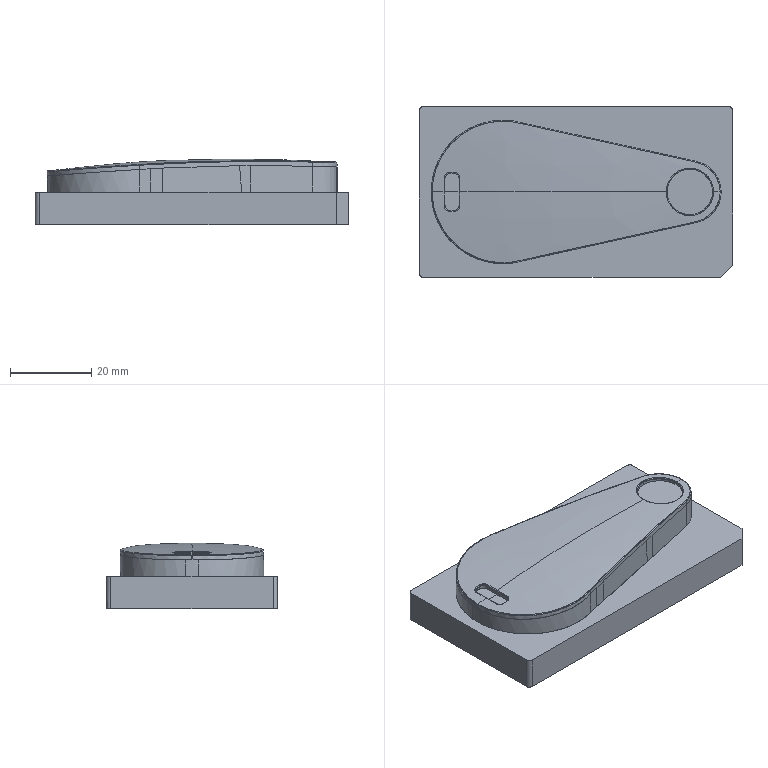NC program | PowerMill | posted with a generic post | part box 77 x 42 x 16.114 mm
Lines 16290 to 17577 of 134652:
N16387 M6
N16388 S18000 M03
N16389 G00 G90 X0.0 Y0.0
N16390 G43 Z9.8037 H28
N16391
N16392 G05 P10000 R4
N16393 X-29.7588 Y2.6569
N16394 Z-1.551
N16395 G01 Z-2.751 F2400.0
N16396 X-29.7423 F4000.0
N16397 G03 X-29.5938 Y2.8054 I0.0 J0.1485
N16398 G01 Y3.0942
N16399 X-29.6282 Y3.438
N16400 X-29.6595 Y3.5057
N16401 X-29.6771 Y3.5369
N16402 X-29.8198 Y3.6917
N16403 X-30.0098 Y3.7818
N16404 X-30.4677 Y3.8359
N16405 X-29.7592 Y2.4875 Z-2.8477
N16406 X-29.7427
N16407 G03 X-29.5942 Y2.636 I0.0 J0.1485
N16408 G01 Y3.0942
N16409 X-29.6289 Y3.438
N16410 X-29.6659 Y3.5172
N16411 X-29.6741 Y3.5316
N16412 X-29.8046 Y3.6727
N16413 X-29.8392 Y3.697
N16414 X-30.0143 Y3.7706
N16415 X-30.6812 Y3.7836
N16416 G00 Z1.579
N16417 G01 X-30.6424 Y-3.6906 F10000.0
N16418 G00 Z-1.551
N16419 G01 Z-2.751 F2400.0
N16420 X-30.6405 Y-3.707 F4000.0
N16421 G03 X-30.4756 Y-3.837 I0.1475 J0.0175
N16422 G01 X-30.0097 Y-3.7818
N16423 X-29.9105 Y-3.7424
N16424 X-29.7524 Y-3.6297
N16425 X-29.7246 Y-3.5995
N16426 X-29.6396 Y-3.4571
N16427 X-29.626 Y-3.4158
N16428 X-29.5938 Y-3.0942
N16429 Y-2.8045
N16430 X-30.8438 Y-3.6168 Z-2.8477
N16431 Y-3.6333
N16432 G03 X-30.6953 Y-3.7818 I0.1485 J0.0
N16433 G01 X-30.1267
N16434 X-29.9315 Y-3.7434
N16435 X-29.8931 Y-3.727
N16436 X-29.7531 Y-3.6281
N16437 X-29.7251 Y-3.598
N16438 X-29.6404 Y-3.4572
N16439 X-29.6265 Y-3.4156
N16440 X-29.5942 Y-3.0942
N16441 Y-2.6348
N16442 X-31.352 Y-3.014 Z-2.7445
N16443 X-31.3523 Y-3.2662 Z-2.7489 F2400.0
N16444 X-31.3304 Y-3.3759 Z-2.7508
N16445 X-31.2927 Y-3.4751 Z-2.7527
N16446 X-31.2617 Y-3.5293 Z-2.7538
N16447 X-31.1326 Y-3.6563 Z-2.7569
N16448 X-31.1088 Y-3.6717 Z-2.7574
N16449 X-30.9361 Y-3.7387 Z-2.7607
N16450 X-30.1396 Y-3.7517 Z-2.7746
N16451 X-29.9375 Y-3.7138 Z-2.7782
N16452 X-29.91 Y-3.7022 Z-2.7787
N16453 X-29.7704 Y-3.6036 Z-2.7817
N16454 X-29.7508 Y-3.5825 Z-2.7822
N16455 X-29.6661 Y-3.4417 Z-2.785
N16456 X-29.6564 Y-3.4127 Z-2.7856
N16457 X-29.6242 Y-3.0927 Z-2.7912
N16458 Y-2.6348 Z-2.7992
N16459 Y-0.7487 Z-2.8321
N16460 X-29.8232 Z-2.8356
N16461 X-30.268 Y-0.8583 Z-2.8435
N16462 X-30.6735 Y-1.0711 Z-2.8515
N16463 X-31.0164 Y-1.3749 Z-2.8595
N16464 X-31.2766 Y-1.7518 Z-2.8675
N16465 X-31.3507 Y-1.9474 Z-2.8712
N16466 X-31.3523 Y-3.2662 Z-2.8942
N16467 X-31.3304 Y-3.3759 Z-2.8961
N16468 X-31.2927 Y-3.4751 Z-2.898
N16469 X-31.2617 Y-3.5293 Z-2.8991
N16470 X-31.1326 Y-3.6563 Z-2.9023
N16471 X-31.1088 Y-3.6717 Z-2.9027
N16472 X-30.9361 Y-3.7387 Z-2.906
N16473 X-30.1396 Y-3.7517 Z-2.9199
N16474 X-29.9375 Y-3.7138 Z-2.9235
N16475 X-29.91 Y-3.7022 Z-2.924
N16476 X-29.7704 Y-3.6036 Z-2.927
N16477 X-29.7508 Y-3.5825 Z-2.9275
N16478 X-29.6661 Y-3.4417 Z-2.9303
N16479 X-29.6564 Y-3.4127 Z-2.9309
N16480 X-29.6242 Y-3.0927 Z-2.9365
N16481 Y-2.6348 Z-2.9445
N16482 X-29.5942
N16483 Y3.0942 F4000.0
N16484 X-29.6289 Y3.438
N16485 X-29.6662 Y3.5178
N16486 X-29.6739 Y3.5314
N16487 X-29.8042 Y3.6723
N16488 X-29.8207 Y3.6866
N16489 X-29.8399 Y3.697
N16490 X-30.0195 Y3.7703
N16491 X-30.9419 Y3.769
N16492 X-31.1184 Y3.7014
N16493 X-31.1367 Y3.6921
N16494 X-31.1527 Y3.6793
N16495 X-31.2857 Y3.5485
N16496 X-31.3653 Y3.3768
N16497 X-31.3723 Y3.3563
N16498 X-31.3746 Y3.3349
N16499 X-31.3823 Y-3.2691
N16500 X-31.3486 Y-3.438
N16501 X-31.2857 Y-3.5478
N16502 X-31.1537 Y-3.6777
N16503 X-31.1378 Y-3.6905
N16504 X-31.1197 Y-3.6997
N16505 X-30.9419 Y-3.7686
N16506 X-30.137 Y-3.7818
N16507 X-29.932 Y-3.7433
N16508 X-29.9114 Y-3.7371
N16509 X-29.8927 Y-3.7267
N16510 X-29.7531 Y-3.6281
N16511 X-29.7376 Y-3.6145
N16512 X-29.7251 Y-3.598
N16513 X-29.6404 Y-3.4572
N16514 X-29.6312 Y-3.4372
N16515 X-29.6266 Y-3.4157
N16516 X-29.5942 Y-3.0942
N16517 Y-2.6348
N16518 X-31.3094 Y-2.9196 Z-2.8412
N16519 Y-3.0928 Z-2.8443 F2400.0
N16520 X-31.2797 Y-3.4125 Z-2.8499
N16521 X-31.27 Y-3.4421 Z-2.8504
N16522 X-31.2008 Y-3.5573 Z-2.8528
N16523 X-31.0441 Y-3.686 Z-2.8563
N16524 X-31.0151 Y-3.7003 Z-2.8569
N16525 X-30.8367 Y-3.7403 Z-2.86
N16526 X-30.1398 Y-3.7518 Z-2.8722
N16527 X-29.9375 Y-3.7138 Z-2.8758
N16528 X-29.91 Y-3.7022 Z-2.8763
N16529 X-29.7704 Y-3.6036 Z-2.8793
N16530 X-29.7508 Y-3.5825 Z-2.8798
N16531 X-29.6661 Y-3.4417 Z-2.8827
N16532 X-29.6564 Y-3.4127 Z-2.8832
N16533 X-29.6242 Y-3.0927 Z-2.8888
N16534 Y-2.6348 Z-2.8968
N16535 Y-0.7487 Z-2.9297
N16536 X-29.8232 Z-2.9332
N16537 X-30.268 Y-0.8583 Z-2.9412
N16538 X-30.6735 Y-1.0711 Z-2.9492
N16539 X-31.0164 Y-1.3749 Z-2.9572
N16540 X-31.2766 Y-1.7518 Z-2.9652
N16541 X-31.3093 Y-1.8381 Z-2.9668
N16542 X-31.3094 Y-3.0928 Z-2.9887
N16543 X-31.2797 Y-3.4125 Z-2.9943
N16544 X-31.27 Y-3.4421 Z-2.9948
N16545 X-31.2008 Y-3.5573 Z-2.9972
N16546 X-31.0441 Y-3.686 Z-3.0007
N16547 X-31.0151 Y-3.7003 Z-3.0013
N16548 X-30.8367 Y-3.7403 Z-3.0045
N16549 X-30.1398 Y-3.7518 Z-3.0166
N16550 X-29.9375 Y-3.7138 Z-3.0202
N16551 X-29.91 Y-3.7022 Z-3.0207
N16552 X-29.7704 Y-3.6036 Z-3.0237
N16553 X-29.7508 Y-3.5825 Z-3.0242
N16554 X-29.6661 Y-3.4417 Z-3.0271
N16555 X-29.6564 Y-3.4127 Z-3.0276
N16556 X-29.6242 Y-3.0927 Z-3.0332
N16557 Y-2.6348 Z-3.0412
N16558 X-29.5942
N16559 Y3.0942 F4000.0
N16560 X-29.6289 Y3.438
N16561 X-29.6665 Y3.5184
N16562 X-29.6738 Y3.5313
N16563 X-29.8042 Y3.6723
N16564 X-29.8207 Y3.6866
N16565 X-29.8398 Y3.697
N16566 X-30.0195 Y3.7703
N16567 X-30.0225 Y3.7704
N16568 X-30.887 Y3.7691
N16569 X-30.9419 Y3.7621
N16570 X-31.1446 Y3.6599
N16571 X-31.2495 Y3.5461
N16572 X-31.3089 Y3.438
N16573 X-31.3389 Y3.2687
N16574 X-31.3394 Y-3.0942
N16575 X-31.3096 Y-3.4153
N16576 X-31.305 Y-3.4372
N16577 X-31.2957 Y-3.4575
N16578 X-31.2238 Y-3.5772
N16579 X-31.0632 Y-3.7092
N16580 X-31.0436 Y-3.7218
N16581 X-31.0216 Y-3.7295
N16582 X-30.8403 Y-3.7703
N16583 X-30.1401 Y-3.7818
N16584 X-30.137
N16585 X-29.9319 Y-3.7433
N16586 X-29.9114 Y-3.7371
N16587 X-29.8927 Y-3.7267
N16588 X-29.7531 Y-3.6281
N16589 X-29.7376 Y-3.6145
N16590 X-29.7251 Y-3.598
N16591 X-29.6404 Y-3.4572
N16592 X-29.6312 Y-3.4372
N16593 X-29.6266 Y-3.4157
N16594 X-29.5942 Y-3.0942
N16595 Y-2.6348
N16596 X-31.3015 Y-2.9085 Z-2.938
N16597 Y-3.0927 Z-2.9412 F2400.0
N16598 X-31.2689 Y-3.4292 Z-2.9471
N16599 X-31.2053 Y-3.5488 Z-2.9495
N16600 X-31.0451 Y-3.6841 Z-2.9531
N16601 X-31.0156 Y-3.6988 Z-2.9537
N16602 X-30.8351 Y-3.7404 Z-2.9569
N16603 X-30.1429 Y-3.7518 Z-2.969
N16604 X-30.1398 Z-2.9691
N16605 X-29.9375 Y-3.7138 Z-2.9727
N16606 X-29.91 Y-3.7022 Z-2.9732
N16607 X-29.7704 Y-3.6036 Z-2.9762
N16608 X-29.7508 Y-3.5825 Z-2.9767
N16609 X-29.6661 Y-3.4417 Z-2.9795
N16610 X-29.6564 Y-3.4127 Z-2.9801
N16611 X-29.6242 Y-3.0927 Z-2.9857
N16612 Y-2.6348 Z-2.9937
N16613 Y-0.7487 Z-3.0266
N16614 X-29.8233 Z-3.0301
N16615 X-30.268 Y-0.8583 Z-3.0381
N16616 X-30.6736 Y-1.0711 Z-3.0461
N16617 X-31.0164 Y-1.3749 Z-3.054
N16618 X-31.2766 Y-1.7518 Z-3.062
N16619 X-31.3015 Y-1.8176 Z-3.0633
N16620 Y-3.0927 Z-3.0855
N16621 X-31.2689 Y-3.4292 Z-3.0914
N16622 X-31.2053 Y-3.5488 Z-3.0938
N16623 X-31.0451 Y-3.6841 Z-3.0974
N16624 X-31.0156 Y-3.6988 Z-3.098
N16625 X-30.8351 Y-3.7404 Z-3.1013
N16626 X-30.1429 Y-3.7518 Z-3.1133
N16627 X-30.1398 Z-3.1134
N16628 X-29.9375 Y-3.7138 Z-3.117
N16629 X-29.91 Y-3.7022 Z-3.1175
N16630 X-29.7704 Y-3.6036 Z-3.1205
N16631 X-29.7508 Y-3.5825 Z-3.121
N16632 X-29.6661 Y-3.4417 Z-3.1239
N16633 X-29.6564 Y-3.4127 Z-3.1244
N16634 X-29.6242 Y-3.0927 Z-3.13
N16635 Y-2.6348 Z-3.138
N16636 X-29.5942
N16637 Y3.0942 F4000.0
N16638 X-29.6289 Y3.438
N16639 X-29.6668 Y3.519
N16640 X-29.6736 Y3.5311
N16641 X-29.8042 Y3.6723
N16642 X-29.8207 Y3.6866
N16643 X-29.8398 Y3.697
N16644 X-30.0195 Y3.7703
N16645 X-30.0256 Y3.7704
N16646 X-30.8858 Y3.7692
N16647 X-30.9419 Y3.7619
N16648 X-31.1261 Y3.6667
N16649 X-31.1447 Y3.6542
N16650 X-31.1601 Y3.6379
N16651 X-31.2696 Y3.4921
N16652 X-31.2824 Y3.4694
N16653 X-31.2889 Y3.4441
N16654 X-31.3315 Y3.0942
N16655 Y-3.0942
N16656 X-31.2982 Y-3.438
N16657 X-31.2291 Y-3.568
N16658 X-31.0644 Y-3.707
N16659 X-31.0446 Y-3.7201
N16660 X-31.0224 Y-3.7281
N16661 X-30.8387 Y-3.7704
N16662 X-30.1431 Y-3.7818
N16663 X-30.1371
N16664 X-29.9319 Y-3.7433
N16665 X-29.9114 Y-3.7371
N16666 X-29.8927 Y-3.7267
N16667 X-29.7531 Y-3.6281
N16668 X-29.7376 Y-3.6145
N16669 X-29.7251 Y-3.598
N16670 X-29.6404 Y-3.4572
N16671 X-29.6312 Y-3.4372
N16672 X-29.6266 Y-3.4157
N16673 X-29.5942 Y-3.0942
N16674 Y-2.6348
N16675 X-31.3014 Y-2.9074 Z-3.0347
N16676 Y-3.0927 Z-3.038 F2400.0
N16677 X-31.2674 Y-3.4293 Z-3.0439
N16678 X-31.2052 Y-3.5489 Z-3.0462
N16679 X-31.045 Y-3.6841 Z-3.0499
N16680 X-31.0156 Y-3.6989 Z-3.0505
N16681 X-30.8349 Y-3.7405 Z-3.0537
N16682 X-30.1459 Y-3.7518 Z-3.0657
N16683 X-30.1399 Z-3.0658
N16684 X-29.9375 Y-3.7138 Z-3.0694
N16685 X-29.91 Y-3.7022 Z-3.07
N16686 X-29.7704 Y-3.6036 Z-3.0729
N16687 X-29.7508 Y-3.5825 Z-3.0734
N16688 X-29.6661 Y-3.4417 Z-3.0763
N16689 X-29.6564 Y-3.4127 Z-3.0768
N16690 X-29.6242 Y-3.0927 Z-3.0825
N16691 Y-2.6348 Z-3.0904
N16692 Y-0.7487 Z-3.1234
N16693 X-29.8233 Z-3.1268
N16694 X-30.268 Y-0.8583 Z-3.1348
N16695 X-30.6736 Y-1.0711 Z-3.1428
N16696 X-31.0164 Y-1.3749 Z-3.1508
N16697 X-31.2766 Y-1.7518 Z-3.1588
N16698 X-31.3014 Y-1.8172 Z-3.16
N16699 Y-3.0927 Z-3.1823
N16700 X-31.2674 Y-3.4293 Z-3.1882
N16701 X-31.2052 Y-3.5489 Z-3.1905
N16702 X-31.045 Y-3.6841 Z-3.1942
N16703 X-31.0156 Y-3.6989 Z-3.1948
N16704 X-30.8349 Y-3.7405 Z-3.198
N16705 X-30.1459 Y-3.7518 Z-3.21
N16706 X-30.1399 Z-3.2101
N16707 X-29.9375 Y-3.7138 Z-3.2137
N16708 X-29.91 Y-3.7022 Z-3.2143
N16709 X-29.7704 Y-3.6036 Z-3.2172
N16710 X-29.7508 Y-3.5825 Z-3.2177
N16711 X-29.6661 Y-3.4417 Z-3.2206
N16712 X-29.6564 Y-3.4127 Z-3.2211
N16713 X-29.6242 Y-3.0927 Z-3.2268
N16714 Y-2.6348 Z-3.2348
N16715 X-29.5942
N16716 Y3.0942 F4000.0
N16717 X-29.629 Y3.438
N16718 X-29.6671 Y3.5196
N16719 X-29.6735 Y3.5309
N16720 X-29.8042 Y3.6723
N16721 X-29.8207 Y3.6866
N16722 X-29.8398 Y3.697
N16723 X-30.0195 Y3.7703
N16724 X-30.0286 Y3.7705
N16725 X-30.8853 Y3.7692
N16726 X-30.9419 Y3.7619
N16727 X-31.126 Y3.6667
N16728 X-31.1446 Y3.6542
N16729 X-31.16 Y3.6379
N16730 X-31.2697 Y3.4916
N16731 X-31.2824 Y3.4689
N16732 X-31.2889 Y3.4437
N16733 X-31.3314 Y3.0942
N16734 Y-3.0942
N16735 X-31.2967 Y-3.438
N16736 X-31.2291 Y-3.568
N16737 X-31.0644 Y-3.7071
N16738 X-31.0446 Y-3.7201
N16739 X-31.0223 Y-3.7281
N16740 X-30.8385 Y-3.7704
N16741 X-30.1462 Y-3.7818
N16742 X-30.1371
N16743 X-29.9319 Y-3.7433
N16744 X-29.9114 Y-3.7371
N16745 X-29.8927 Y-3.7267
N16746 X-29.7531 Y-3.6281
N16747 X-29.7376 Y-3.6145
N16748 X-29.7251 Y-3.598
N16749 X-29.6404 Y-3.4572
N16750 X-29.6312 Y-3.4372
N16751 X-29.6266 Y-3.4157
N16752 X-29.5942 Y-3.0942
N16753 Y-2.6348
N16754 X-31.3014 Y-2.9073 Z-3.1315
N16755 Y-3.0927 Z-3.1347 F2400.0
N16756 X-31.2674 Y-3.4293 Z-3.1406
N16757 X-31.2052 Y-3.5489 Z-3.143
N16758 X-31.045 Y-3.6841 Z-3.1466
N16759 X-31.0156 Y-3.6989 Z-3.1472
N16760 X-30.8346 Y-3.7405 Z-3.1505
N16761 X-30.149 Y-3.7518 Z-3.1624
N16762 X-30.1399 Z-3.1626
N16763 X-29.9375 Y-3.7138 Z-3.1662
N16764 X-29.91 Y-3.7022 Z-3.1667
N16765 X-29.7704 Y-3.6036 Z-3.1697
N16766 X-29.7508 Y-3.5825 Z-3.1702
N16767 X-29.6661 Y-3.4417 Z-3.1731
N16768 X-29.6565 Y-3.4127 Z-3.1736
N16769 X-29.6243 Y-3.0927 Z-3.1792
N16770 Y-2.6348 Z-3.1872
N16771 Y-0.7487 Z-3.2201
N16772 X-29.8233 Z-3.2236
N16773 X-30.268 Y-0.8583 Z-3.2316
N16774 X-30.6736 Y-1.0711 Z-3.2396
N16775 X-31.0164 Y-1.3749 Z-3.2476
N16776 X-31.2766 Y-1.7518 Z-3.2556
N16777 X-31.3014 Y-1.8171 Z-3.2568
N16778 Y-3.0927 Z-3.279
N16779 X-31.2674 Y-3.4293 Z-3.2849
N16780 X-31.2052 Y-3.5489 Z-3.2873
N16781 X-31.045 Y-3.6841 Z-3.291
N16782 X-31.0156 Y-3.6989 Z-3.2915
N16783 X-30.8346 Y-3.7405 Z-3.2948
N16784 X-30.149 Y-3.7518 Z-3.3067
N16785 X-30.1399 Z-3.3069
N16786 X-29.9375 Y-3.7138 Z-3.3105
N16787 X-29.91 Y-3.7022 Z-3.311
N16788 X-29.7704 Y-3.6036 Z-3.314
N16789 X-29.7508 Y-3.5825 Z-3.3145
N16790 X-29.6661 Y-3.4417 Z-3.3174
N16791 X-29.6565 Y-3.4127 Z-3.3179
N16792 X-29.6243 Y-3.0927 Z-3.3235
N16793 Y-2.6348 Z-3.3315
N16794 X-29.5943
N16795 Y3.0942 F4000.0
N16796 X-29.629 Y3.438
N16797 X-29.6674 Y3.5202
N16798 X-29.6733 Y3.5308
N16799 X-29.8042 Y3.6723
N16800 X-29.8207 Y3.6866
N16801 X-29.8398 Y3.697
N16802 X-30.0195 Y3.7703
N16803 X-30.0316 Y3.7705
N16804 X-30.8848 Y3.7693
N16805 X-30.9419 Y3.7619
N16806 X-31.126 Y3.6667
N16807 X-31.1446 Y3.6542
N16808 X-31.1601 Y3.6379
N16809 X-31.2697 Y3.4916
N16810 X-31.2824 Y3.4689
N16811 X-31.2889 Y3.4437
N16812 X-31.3314 Y3.0942
N16813 Y-3.0942
N16814 X-31.2966 Y-3.438
N16815 X-31.2291 Y-3.568
N16816 X-31.0644 Y-3.7071
N16817 X-31.0446 Y-3.7201
N16818 X-31.0223 Y-3.7281
N16819 X-30.8383 Y-3.7705
N16820 X-30.1492 Y-3.7818
N16821 X-30.1371
N16822 X-29.9319 Y-3.7433
N16823 X-29.9114 Y-3.7371
N16824 X-29.8927 Y-3.7267
N16825 X-29.7531 Y-3.6281
N16826 X-29.7376 Y-3.6145
N16827 X-29.7251 Y-3.598
N16828 X-29.6404 Y-3.4572
N16829 X-29.6312 Y-3.4372
N16830 X-29.6266 Y-3.4157
N16831 X-29.5943 Y-3.0942
N16832 Y-2.6348
N16833 X-31.3013 Y-2.9073 Z-3.2283
N16834 Y-3.0927 Z-3.2315 F2400.0
N16835 X-31.2673 Y-3.4293 Z-3.2374
N16836 X-31.2052 Y-3.5489 Z-3.2398
N16837 X-31.045 Y-3.6841 Z-3.2434
N16838 X-31.0156 Y-3.6989 Z-3.244
N16839 X-30.8344 Y-3.7406 Z-3.2472
N16840 X-30.152 Y-3.7518 Z-3.2591
N16841 X-30.1399 Z-3.2594
N16842 X-29.9375 Y-3.7138 Z-3.2629
N16843 X-29.91 Y-3.7021 Z-3.2635
N16844 X-29.7704 Y-3.6036 Z-3.2664
N16845 X-29.7508 Y-3.5825 Z-3.267
N16846 X-29.6661 Y-3.4417 Z-3.2698
N16847 X-29.6565 Y-3.4127 Z-3.2704
N16848 X-29.6243 Y-3.0927 Z-3.276
N16849 Y-2.6348 Z-3.284
N16850 Y-0.7487 Z-3.3169
N16851 X-29.8233 Z-3.3203
N16852 X-30.268 Y-0.8583 Z-3.3283
N16853 X-30.6736 Y-1.0711 Z-3.3363
N16854 X-31.0164 Y-1.3749 Z-3.3443
N16855 X-31.2766 Y-1.7518 Z-3.3523
N16856 X-31.3013 Y-1.817 Z-3.3535
N16857 Y-3.0927 Z-3.3758
N16858 X-31.2673 Y-3.4293 Z-3.3817
N16859 X-31.2052 Y-3.5489 Z-3.3841
N16860 X-31.045 Y-3.6841 Z-3.3877
N16861 X-31.0156 Y-3.6989 Z-3.3883
N16862 X-30.8344 Y-3.7406 Z-3.3915
N16863 X-30.152 Y-3.7518 Z-3.4034
N16864 X-30.1399 Z-3.4037
N16865 X-29.9375 Y-3.7138 Z-3.4073
N16866 X-29.91 Y-3.7021 Z-3.4078
N16867 X-29.7704 Y-3.6036 Z-3.4108
N16868 X-29.7508 Y-3.5825 Z-3.4113
N16869 X-29.6661 Y-3.4417 Z-3.4141
N16870 X-29.6565 Y-3.4127 Z-3.4147
N16871 X-29.6243 Y-3.0927 Z-3.4203
N16872 Y-2.6348 Z-3.4283
N16873 X-29.5943
N16874 Y3.0942 F4000.0
N16875 X-29.629 Y3.438
N16876 X-29.6676 Y3.5208
N16877 X-29.6732 Y3.5306
N16878 X-29.8042 Y3.6723
N16879 X-29.8206 Y3.6866
N16880 X-29.8398 Y3.697
N16881 X-30.0195 Y3.7703
N16882 X-30.0346 Y3.7705
N16883 X-30.8843 Y3.7693
N16884 X-30.9419 Y3.7618
N16885 X-31.126 Y3.6667
N16886 X-31.1446 Y3.6542
N16887 X-31.1601 Y3.6379
N16888 X-31.2697 Y3.4916
N16889 X-31.2824 Y3.4689
N16890 X-31.2889 Y3.4437
N16891 X-31.3314 Y3.0942
N16892 Y-3.0942
N16893 X-31.2966 Y-3.438
N16894 X-31.2291 Y-3.568
N16895 X-31.0644 Y-3.707
N16896 X-31.0446 Y-3.7201
N16897 X-31.0223 Y-3.7281
N16898 X-30.838 Y-3.7705
N16899 X-30.1522 Y-3.7818
N16900 X-30.1371
N16901 X-29.9319 Y-3.7432
N16902 X-29.9114 Y-3.7371
N16903 X-29.8927 Y-3.7267
N16904 X-29.7531 Y-3.6281
N16905 X-29.7376 Y-3.6145
N16906 X-29.7251 Y-3.598
N16907 X-29.6404 Y-3.4572
N16908 X-29.6312 Y-3.4372
N16909 X-29.6266 Y-3.4157
N16910 X-29.5943 Y-3.0942
N16911 Y-2.6348
N16912 X-31.3013 Y-2.9072 Z-3.325
N16913 Y-3.0927 Z-3.3282 F2400.0
N16914 X-31.2673 Y-3.4293 Z-3.3342
N16915 X-31.2052 Y-3.5489 Z-3.3365
N16916 X-31.0451 Y-3.6841 Z-3.3402
N16917 X-31.0156 Y-3.6988 Z-3.3407
N16918 X-30.8341 Y-3.7406 Z-3.344
N16919 X-30.155 Y-3.7518 Z-3.3558
N16920 X-30.1399 Z-3.3561
N16921 X-29.9375 Y-3.7137 Z-3.3597
N16922 X-29.91 Y-3.7021 Z-3.3602
N16923 X-29.7704 Y-3.6036 Z-3.3632
N16924 X-29.7508 Y-3.5825 Z-3.3637
N16925 X-29.6661 Y-3.4417 Z-3.3666
N16926 X-29.6565 Y-3.4127 Z-3.3671
N16927 X-29.6243 Y-3.0927 Z-3.3727
N16928 Y-2.6348 Z-3.3807
N16929 Y-0.7487 Z-3.4136
N16930 X-29.8233 Z-3.4171
N16931 X-30.268 Y-0.8583 Z-3.4251
N16932 X-30.6736 Y-1.0711 Z-3.4331
N16933 X-31.0165 Y-1.3749 Z-3.4411
N16934 X-31.2766 Y-1.7518 Z-3.4491
N16935 X-31.3013 Y-1.8169 Z-3.4503
N16936 Y-3.0927 Z-3.4725
N16937 X-31.2673 Y-3.4293 Z-3.4785
N16938 X-31.2052 Y-3.5489 Z-3.4808
N16939 X-31.0451 Y-3.6841 Z-3.4845
N16940 X-31.0156 Y-3.6988 Z-3.485
N16941 X-30.8341 Y-3.7406 Z-3.4883
N16942 X-30.155 Y-3.7518 Z-3.5001
N16943 X-30.1399 Z-3.5004
N16944 X-29.9375 Y-3.7137 Z-3.504
N16945 X-29.91 Y-3.7021 Z-3.5045
N16946 X-29.7704 Y-3.6036 Z-3.5075
N16947 X-29.7508 Y-3.5825 Z-3.508
N16948 X-29.6661 Y-3.4417 Z-3.5109
N16949 X-29.6565 Y-3.4127 Z-3.5114
N16950 X-29.6243 Y-3.0927 Z-3.517
N16951 Y-2.6348 Z-3.525
N16952 X-29.5943
N16953 Y3.0942 F4000.0
N16954 X-29.629 Y3.438
N16955 X-29.6679 Y3.5214
N16956 X-29.673 Y3.5305
N16957 X-29.8042 Y3.6723
N16958 X-29.8206 Y3.6866
N16959 X-29.8398 Y3.697
N16960 X-30.0195 Y3.7703
N16961 X-30.0377 Y3.7706
N16962 X-30.8838 Y3.7694
N16963 X-30.9419 Y3.7618
N16964 X-31.126 Y3.6667
N16965 X-31.1447 Y3.6542
N16966 X-31.1601 Y3.6378
N16967 X-31.2697 Y3.4916
N16968 X-31.2824 Y3.4689
N16969 X-31.2889 Y3.4437
N16970 X-31.3313 Y3.0942
N16971 Y-3.0942
N16972 X-31.2966 Y-3.438
N16973 X-31.2291 Y-3.568
N16974 X-31.0644 Y-3.707
N16975 X-31.0446 Y-3.7201
N16976 X-31.0223 Y-3.7281
N16977 X-30.8378 Y-3.7706
N16978 X-30.1553 Y-3.7818
N16979 X-30.1371
N16980 X-29.9319 Y-3.7432
N16981 X-29.9114 Y-3.737
N16982 X-29.8927 Y-3.7266
N16983 X-29.7531 Y-3.6281
N16984 X-29.7376 Y-3.6145
N16985 X-29.7251 Y-3.598
N16986 X-29.6404 Y-3.4572
N16987 X-29.6312 Y-3.4372
N16988 X-29.6266 Y-3.4157
N16989 X-29.5943 Y-3.0942
N16990 Y-2.6348
N16991 X-31.3013 Y-2.9072 Z-3.4218
N16992 Y-3.0927 Z-3.425 F2400.0
N16993 X-31.2673 Y-3.4293 Z-3.4309
N16994 X-31.2052 Y-3.5489 Z-3.4333
N16995 X-31.0451 Y-3.6841 Z-3.4369
N16996 X-31.0156 Y-3.6988 Z-3.4375
N16997 X-30.8338 Y-3.7407 Z-3.4408
N16998 X-30.1581 Y-3.7518 Z-3.4525
N16999 X-30.1399 Z-3.4529
N17000 X-29.9375 Y-3.7137 Z-3.4565
N17001 X-29.91 Y-3.7021 Z-3.457
N17002 X-29.7704 Y-3.6036 Z-3.46
N17003 X-29.7508 Y-3.5825 Z-3.4605
N17004 X-29.6662 Y-3.4417 Z-3.4633
N17005 X-29.6565 Y-3.4127 Z-3.4639
N17006 X-29.6243 Y-3.0927 Z-3.4695
N17007 Y-2.6348 Z-3.4775
N17008 Y-0.7487 Z-3.5104
N17009 X-29.8233 Z-3.5139
N17010 X-30.268 Y-0.8583 Z-3.5219
N17011 X-30.6736 Y-1.0711 Z-3.5298
N17012 X-31.0165 Y-1.3749 Z-3.5378
N17013 X-31.2767 Y-1.7518 Z-3.5458
N17014 X-31.3013 Y-1.8168 Z-3.547
N17015 Y-3.0927 Z-3.5693
N17016 X-31.2673 Y-3.4293 Z-3.5752
N17017 X-31.2052 Y-3.5489 Z-3.5776
N17018 X-31.0451 Y-3.6841 Z-3.5812
N17019 X-31.0156 Y-3.6988 Z-3.5818
N17020 X-30.8338 Y-3.7407 Z-3.5851
N17021 X-30.1581 Y-3.7518 Z-3.5968
N17022 X-30.1399 Z-3.5972
N17023 X-29.9375 Y-3.7137 Z-3.6008
N17024 X-29.91 Y-3.7021 Z-3.6013
N17025 X-29.7704 Y-3.6036 Z-3.6043
N17026 X-29.7508 Y-3.5825 Z-3.6048
N17027 X-29.6662 Y-3.4417 Z-3.6076
N17028 X-29.6565 Y-3.4127 Z-3.6082
N17029 X-29.6243 Y-3.0927 Z-3.6138
N17030 Y-2.6348 Z-3.6218
N17031 X-29.5943
N17032 Y3.0942 F4000.0
N17033 X-29.629 Y3.438
N17034 X-29.6682 Y3.522
N17035 X-29.6729 Y3.5303
N17036 X-29.8042 Y3.6723
N17037 X-29.8206 Y3.6866
N17038 X-29.8398 Y3.697
N17039 X-30.0195 Y3.7703
N17040 X-30.0407 Y3.7706
N17041 X-30.8833 Y3.7694
N17042 X-30.9419 Y3.7618
N17043 X-31.126 Y3.6667
N17044 X-31.1447 Y3.6542
N17045 X-31.1601 Y3.6378
N17046 X-31.2697 Y3.4915
N17047 X-31.2824 Y3.4689
N17048 X-31.2889 Y3.4436
N17049 X-31.3313 Y3.0942
N17050 Y-3.0942
N17051 X-31.2966 Y-3.438
N17052 X-31.2291 Y-3.568
N17053 X-31.0644 Y-3.707
N17054 X-31.0446 Y-3.7201
N17055 X-31.0223 Y-3.7281
N17056 X-30.8375 Y-3.7706
N17057 X-30.1583 Y-3.7818
N17058 X-30.1371
N17059 X-29.9319 Y-3.7432
N17060 X-29.9114 Y-3.737
N17061 X-29.8927 Y-3.7266
N17062 X-29.7531 Y-3.6281
N17063 X-29.7376 Y-3.6145
N17064 X-29.7251 Y-3.598
N17065 X-29.6404 Y-3.4572
N17066 X-29.6312 Y-3.4372
N17067 X-29.6266 Y-3.4157
N17068 X-29.5943 Y-3.0942
N17069 Y-2.6348
N17070 G00 Z9.8037
N17071 G05 P0
N17072 (---------------)
N17073 ( END TOOLPATH : 粗公再粗03-外形偏置-D2C )
N17074 (---------------)
N17075
N17076 M05
N17077 G53 Z0.0
N17078 (---------------)
N17079 ( START TOOLPATH : 粗公基准台01-基准面偏置-D10 )
N17080 (---------------)
N17081 ( TOOL NO.    :3 )
N17082 ( TOOL TYPE   : ENDMILL)
N17083 ( TOOL ID     : D10_1_1)
N17084 ( TOOL DIA    : 10.0 LENGTH 71.2)
N17085 T3
N17086 M6
N17087 S8500 M03
N17088 G00 G90 X0.0 Y0.0
N17089 G43 Z9.8037 H3
N17090
N17091 G05 P10000 R8
N17092 X49.125 Y0.9192
N17093 Z-7.11
N17094 G01 Z-8.31 F360.0
N17095 X43.85 F600.0
N17096 X40.8954 Y0.6934
N17097 X40.9107 Y0.2934
N17098 X40.9068 Y-0.4935
N17099 X40.8317 Y-1.4763
N17100 X40.7167 Y-2.2507
N17101 X40.6427 Y-2.6359
N17102 X40.5161 Y-3.1842
N17103 X40.4158 Y-3.5555
N17104 X40.2493 Y-4.0932
N17105 X40.1549 Y-4.3719
N17106 X39.8713 Y-5.0895
N17107 X39.5959 Y-5.6892
N17108 X39.4463 Y-5.9896
N17109 G02 X35.4006 Y-10.5966 I-11.4722 J5.9948
N17110 G01 X37.9432 Y-14.6938
N17111 G02 X39.0409 Y-15.3849 I0.3804 J-0.6131
N17112 G01 X38.8237 Y-17.3818
N17113 G02 X38.7322 Y-17.7998 I-1.9884 J0.2162
N17114 G01 X38.5554 Y-18.3286
N17115 G02 X38.0175 Y-19.1618 I-1.8968 J0.6342
N17116 G01 X36.3968 Y-20.6627
N17117 G02 X35.8562 Y-21.0203 I-1.3589 J1.4674
N17118 G01 X35.2738 Y-21.2814
N17119 G02 X34.4655 Y-21.4564 I-0.8183 J1.825
N17120 G01 X16.7605 Y-21.5445
N17121 G02 X16.6626 Y-20.6678 I-0.0023 J0.4436
N17122 G01 X32.0769 Y-17.2579
N17123 G03 X35.3711 Y-16.1234 I-4.1477 J17.3933
N17124 G01 X35.8782 Y-15.8819
N17125 G03 X37.329 Y-15.075 I-7.7099 J15.5693
N17126 G01 X37.9432 Y-14.6938
N17127 X35.4006 Y-10.5966
N17128 G02 X33.5546 Y-11.6742 I-7.4268 J10.6022
N17129 G02 X32.3896 Y-12.1612 I-5.3362 J11.1282
N17130 G01 X31.872 Y-12.3366
N17131 X31.5065 Y-12.4458
N17132 X30.7667 Y-12.6341
N17133 X-11.6587 Y-21.9988
N17134 X-12.2125 Y-22.1507
N17135 X-12.9152 Y-22.321
N17136 G02 X-14.4601 Y-22.6141 I-5.1927 J23.1506
N17137 G01 X-15.5136 Y-22.7516
N17138 X-16.3314 Y-22.8242
N17139 G02 X-19.2196 Y-22.8467 I-1.6196 J22.5037
N17140 G01 X-20.0204 Y-22.7879
N17141 X-20.8266 Y-22.7003
N17142 X-21.6623 Y-22.5784
N17143 X-22.4972 Y-22.4254
N17144 X-23.2427 Y-22.2617
N17145 X-24.0587 Y-22.0525
N17146 X-24.4109 Y-21.951
N17147 X-25.4174 Y-21.6303
N17148 X-26.3495 Y-21.2846
N17149 X-26.9672 Y-21.0305
N17150 X-27.5358 Y-20.7776
N17151 G02 X-28.8763 Y-20.1046 I9.0451 J19.6881
N17152 G01 X-29.6516 Y-19.6635
N17153 X-30.353 Y-19.2298
N17154 X-31.0964 Y-18.7297
N17155 X-32.0626 Y-18.0128
N17156 X-32.8425 Y-17.372
N17157 X-33.4364 Y-16.8457
N17158 X-33.8843 Y-16.4222
N17159 X-37.256 Y-19.8378
N17160 X-36.5256 Y-20.5588
N17161 G02 X-37.1164 Y-21.5516 I-0.4167 J-0.4242
N17162 G01 X-37.6537 Y-21.3871
N17163 G02 X-38.4375 Y-20.7791 I0.4095 J1.3372
N17164 G01 X-38.6369 Y-20.4527
N17165 X-38.9641 Y-19.8413
N17166 G02 X-37.9864 Y-19.1168 I0.5437 J0.2883
N17167 G01 X-37.256 Y-19.8378
N17168 X-33.8843 Y-16.4222
N17169 X-34.2399 Y-16.0697
N17170 X-34.7059 Y-15.5832
N17171 G02 X-36.4624 Y-13.4493 I16.4302 J15.314
N17172 G01 X-36.9486 Y-12.7532
N17173 G02 X-38.6269 Y-9.8018 I18.8644 J12.6798
N17174 G01 X-38.8933 Y-9.219
N17175 X-39.0725 Y-8.8019
N17176 X-39.2422 Y-8.3809
N17177 X-39.5283 Y-7.6142
N17178 G02 X-40.7562 Y-1.8623 I21.4848 J7.5936
N17179 G01 X-40.8154 Y-0.8756
N17180 X-40.8319 Y0.1135
N17181 X-40.8056 Y1.1023
N17182 X-40.7562 Y1.8623
N17183 G02 X-39.5283 Y7.6142 I22.7145 J-1.8421
N17184 G01 X-39.2422 Y8.3809
N17185 X-39.0725 Y8.8019
N17186 X-38.8933 Y9.219
N17187 X-38.6269 Y9.8018
N17188 G02 X-36.9486 Y12.7532 I20.6129 J-9.7683
N17189 G01 X-36.4624 Y13.4493
N17190 G02 X-34.7059 Y15.5832 I18.1864 J-13.1799
N17191 G01 X-34.5536 Y15.7422
N17192 X-37.9789 Y19.1112
N17193 G02 X-38.9904 Y19.7286 I-0.4363 J0.4225
N17194 G01 X-38.8127 Y20.2533
N17195 G02 X-38.4983 Y20.7576 I1.2296 J-0.4164
N17196 G01 X-38.2511 Y21.0034
N17197 G02 X-37.7439 Y21.3151 I0.9153 J-0.9207
N17198 G01 X-37.1822 Y21.5011
N17199 G02 X-36.5763 Y20.4932 I0.1895 J-0.5722
N17200 G01 X-37.4059 Y19.6938
N17201 X-37.9789 Y19.1112
N17202 X-34.5536 Y15.7422
N17203 X-34.2399 Y16.0697
N17204 G02 X-32.8425 Y17.372 I15.7853 J-15.5376
N17205 G01 X-31.966 Y18.0881
N17206 X-31.0964 Y18.7297
N17207 G02 X-29.6516 Y19.6635 I12.7792 J-18.1865
N17208 G01 X-28.8763 Y20.1046
N17209 G02 X-27.5358 Y20.7776 I10.4499 J-19.1432
N17210 G01 X-26.6596 Y21.1604
N17211 X-25.6951 Y21.5314
N17212 X-25.1378 Y21.7237
N17213 X-24.2706 Y21.9927
N17214 X-23.9255 Y22.0882
N17215 X-23.2427 Y22.2617
N17216 X-22.4972 Y22.4254
N17217 X-21.4457 Y22.6134
N17218 X-20.6435 Y22.7227
N17219 X-19.8372 Y22.8039
N17220 X-19.0092 Y22.8581
N17221 G02 X-16.3314 Y22.8242 I1.0521 J-22.6807
N17222 G01 X-15.2705 Y22.7243
N17223 X-14.1428 Y22.5641
N17224 X-13.1242 Y22.3672
N17225 X-12.2125 Y22.1507
N17226 X-11.6587 Y21.9988
N17227 X15.6188 Y15.9774
N17228 X16.6535 Y20.6689
N17229 G02 X16.7531 Y21.5458 I0.0956 J0.4332
N17230 G01 X36.9031 Y21.3638
N17231 G02 X39.0141 Y19.2489 I-0.0192 J-2.1302
N17232 G01 X39.0424 Y15.3053
N17233 G02 X37.9355 Y14.695 I-0.7188 J-0.0052
N17234 G01 X37.609 Y14.9043
N17235 G03 X31.7422 Y17.3409 I-9.7618 J-15.2232
N17236 G01 X16.6535 Y20.6689
N17237 X15.6188 Y15.9774
N17238 X30.8431 Y12.6167
N17239 G02 X34.4311 Y11.2118 I-2.8536 J-12.5722
N17240 G01 X34.909 Y10.923
N17241 X35.2284 Y10.7137
N17242 X35.6836 Y10.3913
N17243 X35.971 Y10.1725
N17244 X36.3548 Y9.8589
N17245 X36.8729 Y9.3931
N17246 X37.1284 Y9.147
N17247 G02 X39.7068 Y5.4591 I-9.1411 J-9.1361
N17248 G02 X40.5993 Y2.8416 I-11.6134 J-5.421
N17249 G01 X40.663 Y2.5471
N17250 X40.7167 Y2.2506
N17251 X40.8318 Y1.4763
N17252 X40.8954 Y0.6934
N17253 X43.85 Y0.9192
N17254 G00 Z9.8037
N17255 G05 P0
N17256 (---------------)
N17257 ( END TOOLPATH : 粗公基准台01-基准面偏置-D10 )
N17258 (---------------)
N17259 ( START TOOLPATH : 粗公基准台01-外形侧光-D10 )
N17260 (---------------)
N17261 G00 X0.0 Y0.0 Z10.803
N17262 G05 P10000 R8
N17263 X25.2831 Y-13.9156
N17264 Z-7.08
N17265 G01 Z-8.28 F360.0
N17266 G03 X24.1527 Y-13.7152 I-0.8071 J-1.2644 F600.0
N17267 G01 X-11.7342 Y-21.637
N17268 G02 X-22.0863 Y22.1291 I-6.217 J21.6368
N17269 G02 X-11.7267 Y21.6349 I4.1361 J-22.124
N17270 G01 X9.4398 Y16.9628
N17271 X30.6089 Y12.2901
N17272 G02 X40.545 Y-0.0039 I-2.6328 J-12.2901
N17273 G02 X30.6083 Y-12.2902 I-12.5689 J0.0039
N17274 G01 X24.1527 Y-13.7152
N17275 G03 X23.2117 Y-14.3729 I0.3233 J-1.4648
N17276 G01 X25.1792 Y-13.8566
N17277 G03 X24.0487 Y-13.6562 I-0.8071 J-1.2643
N17278 G01 X-11.7459 Y-21.5572
N17279 G02 X-22.072 Y22.0504 I-6.2052 J21.557
N17280 G02 X-11.7459 Y21.5572 I4.1219 J-22.046
N17281 G01 X9.4226 Y16.8847
N17282 X30.591 Y12.2121
N17283 G02 X40.465 Y-0.0039 I-2.6149 J-12.2121
N17284 G02 X30.591 Y-12.2121 I-12.4889 J0.0039
N17285 G01 X24.0487 Y-13.6562
N17286 G03 X23.1077 Y-14.3138 I0.3234 J-1.4647
N17287 G00 Z10.803
N17288 G05 P0
N17289 (---------------)
N17290 ( END TOOLPATH : 粗公基准台01-外形侧光-D10 )
N17291 (---------------)
N17292 ( START TOOLPATH : 粗公基准台01-基准台侧光-D10 )
N17293 (---------------)
N17294 G00 X0.0 Y0.0 Z9.8037
N17295 G05 P10000 R8
N17296 X43.4716 Y-27.2827
N17297 Z-15.01
N17298 G01 Z-16.21 F360.0
N17299 G03 X39.9355 Y-23.7478 I-1.7681 J1.7675 F600.0
N17300 G01 X39.0428 Y-24.6408
N17301 X39.0411 Y-24.6424
N17302 X39.0395 Y-24.6439
N17303 X38.7175 Y-24.9311
N17304 X38.7154 Y-24.9329
N17305 X38.7132 Y-24.9347
N17306 X38.5069 Y-25.0944
N17307 X38.5052 Y-25.0958
N17308 X38.5034 Y-25.0971
N17309 X38.2627 Y-25.2631
N17310 X38.26 Y-25.2648
N17311 X38.2572 Y-25.2665
N17312 X37.8102 Y-25.5242
N17313 X37.8067 Y-25.5261
N17314 X37.8031 Y-25.5278
N17315 X37.3561 Y-25.7287
N17316 X37.3525 Y-25.7302
N17317 X37.3489 Y-25.7315
N17318 X36.9019 Y-25.8827
N17319 X36.8981 Y-25.8838
N17320 X36.8942 Y-25.8848
N17321 X36.3798 Y-26.0031
N17322 X36.3762 Y-26.0039
N17323 X36.3726 Y-26.0044
N17324 X35.9931 Y-26.056
N17325 X35.9898 Y-26.0563
N17326 X35.9865 Y-26.0566
N17327 X35.5395 Y-26.0798
N17328 X35.5374
N17329 X35.5354 Y-26.0799
N17330 X-37.3233 Y-26.08
N17331 X-37.324
N17332 X-37.3246
N17333 X-37.7716 Y-26.0727
N17334 X-37.7742 Y-26.0726
N17335 X-37.7767 Y-26.0724
N17336 X-38.2237 Y-26.0364
N17337 X-38.2267 Y-26.0361
N17338 X-38.2298 Y-26.0356
N17339 X-38.6767 Y-25.965
N17340 X-38.6798 Y-25.9645
N17341 X-38.6828 Y-25.9638
N17342 X-39.1298 Y-25.857
N17343 X-39.1329 Y-25.8563
N17344 X-39.1358 Y-25.8553
N17345 X-39.5828 Y-25.7109
N17346 X-39.5855 Y-25.71
N17347 X-39.5882 Y-25.709
N17348 X-39.9762 Y-25.5524
N17349 X-39.9794 Y-25.551
N17350 X-39.9825 Y-25.5495
N17351 X-40.4884 Y-25.2925
N17352 X-40.4909 Y-25.2912
N17353 X-40.4934 Y-25.2898
N17354 X-40.8101 Y-25.0998
N17355 X-40.8118 Y-25.0988
N17356 X-40.8134 Y-25.0977
N17357 X-40.9436 Y-25.0107
N17358 X-40.9458 Y-25.0092
N17359 X-40.9479 Y-25.0076
N17360 X-41.3949 Y-24.6643
N17361 X-41.3976 Y-24.6621
N17362 X-41.4002 Y-24.6598
N17363 X-41.8472 Y-24.2504
N17364 X-41.8505 Y-24.2472
N17365 X-41.8535 Y-24.2439
N17366 X-42.3005 Y-23.7294
N17367 X-42.303 Y-23.7264
N17368 X-42.3054 Y-23.7232
N17369 X-42.6129 Y-23.2895
N17370 X-42.6149 Y-23.2866
N17371 X-42.6168 Y-23.2835
N17372 X-42.8772 Y-22.8365
N17373 X-42.8788 Y-22.8336
N17374 X-42.8803 Y-22.8307
N17375 X-43.0932 Y-22.3837
N17376 X-43.0945 Y-22.3807
N17377 X-43.0957 Y-22.3776
N17378 X-43.2649 Y-21.9306
N17379 X-43.266 Y-21.9276
N17380 X-43.2669 Y-21.9245
N17381 X-43.3962 Y-21.4775
N17382 X-43.397 Y-21.4748
N17383 X-43.3976 Y-21.4719
N17384 X-43.4926 Y-21.025
N17385 X-43.4932 Y-21.0218
N17386 X-43.4937 Y-21.0186
N17387 X-43.5515 Y-20.5716
N17388 X-43.5518 Y-20.5688
N17389 X-43.552 Y-20.5661
N17390 X-43.5786 Y-20.1191
N17391 X-43.5787 Y-20.1168
N17392 Y-20.1146
N17393 X-43.58 Y-19.6676
N17394 Y-19.6675
N17395 Y-19.6674
N17396 Y19.2204
N17397 Y19.2205
N17398 X-43.5787 Y20.1145
N17399 Y20.1168
N17400 X-43.5786 Y20.1191
N17401 X-43.552 Y20.5661
N17402 X-43.5518 Y20.5688
N17403 X-43.5515 Y20.5716
N17404 X-43.4937 Y21.0186
N17405 X-43.4932 Y21.0218
N17406 X-43.4926 Y21.025
N17407 X-43.3976 Y21.4719
N17408 X-43.397 Y21.4748
N17409 X-43.3962 Y21.4775
N17410 X-43.2669 Y21.9245
N17411 X-43.266 Y21.9276
N17412 X-43.2649 Y21.9306
N17413 X-43.0957 Y22.3776
N17414 X-43.0945 Y22.3807
N17415 X-43.0932 Y22.3837
N17416 X-42.8803 Y22.8307
N17417 X-42.8788 Y22.8336
N17418 X-42.8772 Y22.8365
N17419 X-42.6168 Y23.2835
N17420 X-42.6149 Y23.2866
N17421 X-42.6129 Y23.2895
N17422 X-42.3054 Y23.7232
N17423 X-42.3032 Y23.7262
N17424 X-42.3008 Y23.729
N17425 X-41.9057 Y24.1893
N17426 X-41.9027 Y24.1926
N17427 X-41.8996 Y24.1957
N17428 X-41.4204 Y24.6427
N17429 X-41.4176 Y24.6452
N17430 X-41.4147 Y24.6476
N17431 X-40.948 Y25.0075
N17432 X-40.9459 Y25.0091
N17433 X-40.9436 Y25.0107
N17434 X-40.8134 Y25.0977
N17435 X-40.8118 Y25.0988
N17436 X-40.8101 Y25.0998
N17437 X-40.4934 Y25.2898
N17438 X-40.4911 Y25.2911
N17439 X-40.4888 Y25.2923
N17440 X-40.0419 Y25.5227
N17441 X-40.0387 Y25.5242
N17442 X-40.0356 Y25.5256
N17443 X-39.5886 Y25.7088
N17444 X-39.5857 Y25.71
N17445 X-39.5828 Y25.7109
N17446 X-39.1358 Y25.8554
N17447 X-39.1329 Y25.8563
N17448 X-39.1298 Y25.857
N17449 X-38.6828 Y25.9638
N17450 X-38.6798 Y25.9645
N17451 X-38.6767 Y25.965
N17452 X-38.2298 Y26.0356
N17453 X-38.2267 Y26.0361
N17454 X-38.2237 Y26.0364
N17455 X-37.7767 Y26.0724
N17456 X-37.7742 Y26.0726
N17457 X-37.7716 Y26.0727
N17458 X-37.3246 Y26.08
N17459 X-37.324
N17460 X-37.3233
N17461 X0.0
N17462 X37.3233
N17463 X37.324
N17464 X37.3246
N17465 X37.7716 Y26.0727
N17466 X37.7742 Y26.0726
N17467 X37.7767 Y26.0724
N17468 X38.2237 Y26.0364
N17469 X38.2267 Y26.0361
N17470 X38.2298 Y26.0356
N17471 X38.6767 Y25.965
N17472 X38.6798 Y25.9645
N17473 X38.6828 Y25.9638
N17474 X39.1298 Y25.857
N17475 X39.1329 Y25.8563
N17476 X39.1358 Y25.8553
N17477 X39.5828 Y25.7109
N17478 X39.5855 Y25.71
N17479 X39.5882 Y25.709
N17480 X39.9762 Y25.5524
N17481 X39.9794 Y25.551
N17482 X39.9825 Y25.5495
N17483 X40.4884 Y25.2925
N17484 X40.4909 Y25.2912
N17485 X40.4934 Y25.2898
N17486 X40.8101 Y25.0998
N17487 X40.8118 Y25.0988
N17488 X40.8134 Y25.0977
N17489 X40.9436 Y25.0107
N17490 X40.9458 Y25.0092
N17491 X40.9479 Y25.0076
N17492 X41.3949 Y24.6643
N17493 X41.3976 Y24.6621
N17494 X41.4002 Y24.6598
N17495 X41.8472 Y24.2504
N17496 X41.8505 Y24.2472
N17497 X41.8535 Y24.2439
N17498 X42.3005 Y23.7294
N17499 X42.303 Y23.7264
N17500 X42.3054 Y23.7232
N17501 X42.6129 Y23.2895
N17502 X42.6149 Y23.2866
N17503 X42.6168 Y23.2835
N17504 X42.8772 Y22.8365
N17505 X42.8788 Y22.8336
N17506 X42.8803 Y22.8307
N17507 X43.0932 Y22.3837
N17508 X43.0945 Y22.3807
N17509 X43.0958 Y22.3776
N17510 X43.2649 Y21.9306
N17511 X43.266 Y21.9276
N17512 X43.267 Y21.9245
N17513 X43.3962 Y21.4775
N17514 X43.397 Y21.4748
N17515 X43.3976 Y21.4719
N17516 X43.4926 Y21.025
N17517 X43.4932 Y21.0218
N17518 X43.4937 Y21.0186
N17519 X43.5514 Y20.5716
N17520 X43.5518 Y20.5688
N17521 X43.552 Y20.5661
N17522 X43.5786 Y20.1191
N17523 X43.5787 Y20.1168
N17524 Y20.1146
N17525 X43.58 Y19.6676
N17526 Y19.6675
N17527 Y19.6674
N17528 Y-17.8794
N17529 Y-17.8804
N17530 Y-17.8813
N17531 X43.5694 Y-18.3283
N17532 X43.5692 Y-18.3318
N17533 X43.5689 Y-18.3352
N17534 X43.5194 Y-18.7822
N17535 X43.5189 Y-18.7858
N17536 X43.5182 Y-18.7894
N17537 X43.4272 Y-19.2364
N17538 X43.4264 Y-19.24
N17539 X43.4254 Y-19.2435
N17540 X43.2904 Y-19.6905
N17541 X43.2896 Y-19.6931
N17542 X43.2886 Y-19.6957
N17543 X43.2089 Y-19.9059
N17544 X43.2082 Y-19.9077
N17545 X43.2075 Y-19.9095
N17546 X43.1043 Y-20.1463
N17547 X43.103 Y-20.1491
N17548 X43.1017 Y-20.1518
N17549 X42.8648 Y-20.5988
N17550 X42.8635 Y-20.6013
N17551 X42.862 Y-20.6037
N17552 X42.755 Y-20.7751
N17553 X42.7538 Y-20.7769
N17554 X42.7526 Y-20.7787
N17555 X42.5592 Y-21.0543
N17556 X42.5575 Y-21.0567
N17557 X42.5557 Y-21.059
N17558 X42.3021 Y-21.369
N17559 X42.3006 Y-21.3708
N17560 X42.299 Y-21.3726
N17561 X42.1728 Y-21.5095
N17562 X42.1717 Y-21.5107
N17563 X42.1706 Y-21.5119
N17564 X39.9355 Y-23.7478
N17565 G03 X43.4716 Y-27.2827 I1.768 J-1.7674
N17566 G01 X43.4202 Y-27.221
N17567 G03 X39.884 Y-23.6861 I-1.7681 J1.7675
N17568 G01 X38.9862 Y-24.5842
N17569 X38.6643 Y-24.8714
N17570 X38.458 Y-25.0312
N17571 X38.2173 Y-25.1972
N17572 X37.7703 Y-25.4549
N17573 X37.3233 Y-25.6557
N17574 X36.8763 Y-25.8069
N17575 X36.3619 Y-25.9252
N17576 X35.9823 Y-25.9767
N17577 X35.5354 Y-25.9999
N17578 X-37.3233 Y-26.0
N17579 X-37.7703 Y-25.9927
N17580 X-38.2173 Y-25.9566
N17581 X-38.6643 Y-25.886
N17582 X-39.1112 Y-25.7792
N17583 X-39.5582 Y-25.6348
N17584 X-39.9463 Y-25.4782
N17585 X-40.4522 Y-25.2212
N17586 X-40.769 Y-25.0312
N17587 X-40.8992 Y-24.9441
N17588 X-41.3462 Y-24.6009
N17589 X-41.7932 Y-24.1914
N17590 X-42.2401 Y-23.6769
N17591 X-42.5477 Y-23.2433
N17592 X-42.8081 Y-22.7963
N17593 X-43.0209 Y-22.3493
N17594 X-43.1901 Y-21.9023
N17595 X-43.3194 Y-21.4553
N17596 X-43.4143 Y-21.0083
N17597 X-43.4721 Y-20.5613
N17598 X-43.4987 Y-20.1144
N17599 X-43.5 Y-19.6674
N17600 Y19.2204
N17601 X-43.4987 Y20.1144
N17602 X-43.4721 Y20.5613
N17603 X-43.4143 Y21.0083
N17604 X-43.3194 Y21.4553
N17605 X-43.1901 Y21.9023
N17606 X-43.0209 Y22.3493
N17607 X-42.8081 Y22.7963
N17608 X-42.5477 Y23.2433
N17609 X-42.2401 Y23.6769
N17610 X-41.845 Y24.1372
N17611 X-41.3658 Y24.5842
N17612 X-40.8992 Y24.9441
N17613 X-40.769 Y25.0312
N17614 X-40.4522 Y25.2212
N17615 X-40.0052 Y25.4515
N17616 X-39.5582 Y25.6348
N17617 X-39.1112 Y25.7792
N17618 X-38.6643 Y25.886
N17619 X-38.2173 Y25.9566
N17620 X-37.7703 Y25.9927
N17621 X-37.3233 Y26.0
N17622 X0.0
N17623 X37.3233
N17624 X37.7703 Y25.9927
N17625 X38.2173 Y25.9566
N17626 X38.6643 Y25.886
N17627 X39.1112 Y25.7792
N17628 X39.5582 Y25.6348
N17629 X39.9463 Y25.4782
N17630 X40.4522 Y25.2212
N17631 X40.769 Y25.0312
N17632 X40.8992 Y24.9441
N17633 X41.3462 Y24.6009
N17634 X41.7932 Y24.1914
N17635 X42.2401 Y23.6769
N17636 X42.5477 Y23.2433
N17637 X42.8081 Y22.7963
N17638 X43.0209 Y22.3493
N17639 X43.1901 Y21.9023
N17640 X43.3194 Y21.4553
N17641 X43.4144 Y21.0083
N17642 X43.4721 Y20.5613
N17643 X43.4987 Y20.1144
N17644 X43.5 Y19.6674
N17645 Y-17.8794
N17646 X43.4894 Y-18.3264
N17647 X43.4399 Y-18.7734
N17648 X43.3488 Y-19.2204
N17649 X43.2138 Y-19.6674
N17650 X43.1341 Y-19.8775
N17651 X43.031 Y-20.1144
N17652 X42.7941 Y-20.5613
N17653 X42.6871 Y-20.7328
N17654 X42.4937 Y-21.0083
N17655 X42.2401 Y-21.3184
N17656 X42.114 Y-21.4553
N17657 X39.884 Y-23.6861
N17658 G03 X43.4202 Y-27.221 I1.7681 J-1.7674
N17659 G00 Z9.8037
N17660 G05 P0
N17661 (---------------)
N17662 ( END TOOLPATH : 粗公基准台01-基准台侧光-D10 )
N17663 (---------------)
N17664
N17665 M05
N17666 G53 Z0.0
N17667 (---------------)
N17668 ( START TOOLPATH : 粗公精光01-平行-R2 )
N17669 (---------------)
N17670 ( TOOL NO.    :7 )
N17671 ( TOOL TYPE   : BALLNOSED)
N17672 ( TOOL ID     : R2_2_1)
N17673 ( TOOL DIA    : 4.0 LENGTH 60.4)
N17674 T7